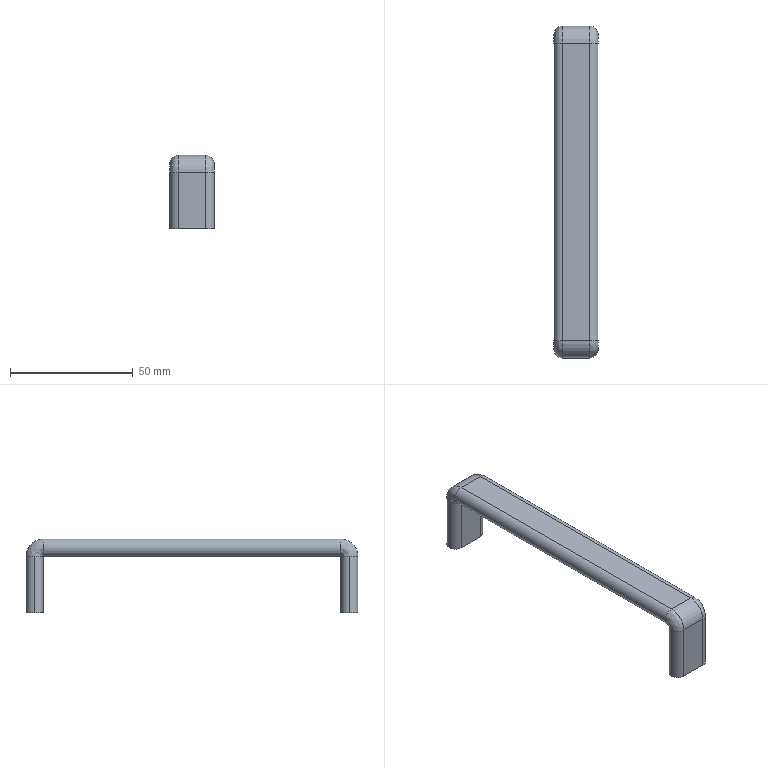Part | SolidWorks | features BaseBody 1 | 1 solid | 30 faces | box 18 x 135 x 30 mm | volume 20354 mm3 | cylinder 14 | plane 8 | cone 4 | spline 4 | commonest cylinder face diameters 7 x8 3.3 x4 14 x2
STEP:
#1=CARTESIAN_POINT('',(-9.,-64.,23.));
#2=VERTEX_POINT('',#1);
#3=CARTESIAN_POINT('',(-5.5,-67.5,23.));
#4=VERTEX_POINT('',#3);
#5=CARTESIAN_POINT('',(-5.5,-64.,23.));
#6=DIRECTION('',(0.,0.,1.));
#7=DIRECTION('',(0.,-1.,0.));
#8=AXIS2_PLACEMENT_3D('',#5,#6,#7);
#9=CIRCLE('',#8,3.5);
#10=EDGE_CURVE('',#2,#4,#9,.T.);
#11=ORIENTED_EDGE('',*,*,#10,.F.);
#12=CARTESIAN_POINT('',(-9.,-64.,0.));
#13=VERTEX_POINT('',#12);
#14=CARTESIAN_POINT('',(-9.,-64.,23.));
#15=DIRECTION('',(0.,0.,-1.));
#16=VECTOR('',#15,1000.);
#17=LINE('',#14,#16);
#18=EDGE_CURVE('',#2,#13,#17,.T.);
#19=ORIENTED_EDGE('',*,*,#18,.T.);
#20=CARTESIAN_POINT('',(-5.5,-67.5,0.));
#21=VERTEX_POINT('',#20);
#22=CARTESIAN_POINT('',(-5.5,-64.,0.));
#23=DIRECTION('',(0.,0.,1.));
#24=DIRECTION('',(-1.,0.,0.));
#25=AXIS2_PLACEMENT_3D('',#22,#23,#24);
#26=CIRCLE('',#25,3.5);
#27=EDGE_CURVE('',#13,#21,#26,.T.);
#28=ORIENTED_EDGE('',*,*,#27,.T.);
#29=CARTESIAN_POINT('',(-5.5,-67.5,23.));
#30=DIRECTION('',(0.,0.,1.));
#31=VECTOR('',#30,1000.);
#32=LINE('',#29,#31);
#33=EDGE_CURVE('',#21,#4,#32,.T.);
#34=ORIENTED_EDGE('',*,*,#33,.T.);
#35=EDGE_LOOP('',(#11,#19,#28,#34));
#36=FACE_OUTER_BOUND('',#35,.T.);
#37=CARTESIAN_POINT('',(-5.5,-64.,23.));
#38=DIRECTION('',(0.,0.,-1.));
#39=DIRECTION('',(-1.,0.,0.));
#40=AXIS2_PLACEMENT_3D('',#37,#38,#39);
#41=CYLINDRICAL_SURFACE('',#40,3.5);
#42=ADVANCED_FACE('',(#36),#41,.T.);
#43=CARTESIAN_POINT('',(-9.,64.,23.));
#44=VERTEX_POINT('',#43);
#45=CARTESIAN_POINT('',(-5.5,60.5,23.));
#46=VERTEX_POINT('',#45);
#47=CARTESIAN_POINT('',(-5.5,64.,23.));
#48=DIRECTION('',(0.,0.,1.));
#49=DIRECTION('',(0.,1.,0.));
#50=AXIS2_PLACEMENT_3D('',#47,#48,#49);
#51=CIRCLE('',#50,3.5);
#52=EDGE_CURVE('',#44,#46,#51,.T.);
#53=ORIENTED_EDGE('',*,*,#52,.F.);
#54=CARTESIAN_POINT('',(-9.,64.,0.));
#55=VERTEX_POINT('',#54);
#56=CARTESIAN_POINT('',(-9.,64.,23.));
#57=DIRECTION('',(0.,0.,-1.));
#58=VECTOR('',#57,1000.);
#59=LINE('',#56,#58);
#60=EDGE_CURVE('',#44,#55,#59,.T.);
#61=ORIENTED_EDGE('',*,*,#60,.T.);
#62=CARTESIAN_POINT('',(-5.5,60.5,0.));
#63=VERTEX_POINT('',#62);
#64=CARTESIAN_POINT('',(-5.5,64.,0.));
#65=DIRECTION('',(0.,0.,1.));
#66=DIRECTION('',(-1.,0.,0.));
#67=AXIS2_PLACEMENT_3D('',#64,#65,#66);
#68=CIRCLE('',#67,3.5);
#69=EDGE_CURVE('',#55,#63,#68,.T.);
#70=ORIENTED_EDGE('',*,*,#69,.T.);
#71=CARTESIAN_POINT('',(-5.5,60.5,23.));
#72=DIRECTION('',(0.,0.,1.));
#73=VECTOR('',#72,1000.);
#74=LINE('',#71,#73);
#75=EDGE_CURVE('',#63,#46,#74,.T.);
#76=ORIENTED_EDGE('',*,*,#75,.T.);
#77=EDGE_LOOP('',(#53,#61,#70,#76));
#78=FACE_OUTER_BOUND('',#77,.T.);
#79=CARTESIAN_POINT('',(-5.5,64.,23.));
#80=DIRECTION('',(0.,0.,-1.));
#81=DIRECTION('',(-1.,0.,0.));
#82=AXIS2_PLACEMENT_3D('',#79,#80,#81);
#83=CYLINDRICAL_SURFACE('',#82,3.5);
#84=ADVANCED_FACE('',(#78),#83,.T.);
#85=CARTESIAN_POINT('',(1.65,-64.,11.5));
#86=VERTEX_POINT('',#85);
#87=CARTESIAN_POINT('',(-1.65,-64.,11.5));
#88=VERTEX_POINT('',#87);
#89=CARTESIAN_POINT('',(0.,-64.,11.5));
#90=DIRECTION('',(0.,0.,-1.));
#91=DIRECTION('',(-1.,0.,0.));
#92=AXIS2_PLACEMENT_3D('',#89,#90,#91);
#93=CIRCLE('',#92,1.65);
#94=EDGE_CURVE('',#86,#88,#93,.T.);
#95=ORIENTED_EDGE('',*,*,#94,.F.);
#96=CARTESIAN_POINT('',(1.65,-64.,0.));
#97=VERTEX_POINT('',#96);
#98=CARTESIAN_POINT('',(1.65,-64.,0.));
#99=DIRECTION('',(0.,0.,-1.));
#100=VECTOR('',#99,1000.);
#101=LINE('',#98,#100);
#102=EDGE_CURVE('',#86,#97,#101,.T.);
#103=ORIENTED_EDGE('',*,*,#102,.T.);
#104=CARTESIAN_POINT('',(-1.65,-64.,0.));
#105=VERTEX_POINT('',#104);
#106=CARTESIAN_POINT('',(0.,-64.,0.));
#107=DIRECTION('',(0.,0.,1.));
#108=DIRECTION('',(-1.,0.,0.));
#109=AXIS2_PLACEMENT_3D('',#106,#107,#108);
#110=CIRCLE('',#109,1.65);
#111=EDGE_CURVE('',#105,#97,#110,.T.);
#112=ORIENTED_EDGE('',*,*,#111,.F.);
#113=CARTESIAN_POINT('',(-1.65,-64.,0.));
#114=DIRECTION('',(0.,0.,-1.));
#115=VECTOR('',#114,1000.);
#116=LINE('',#113,#115);
#117=EDGE_CURVE('',#88,#105,#116,.T.);
#118=ORIENTED_EDGE('',*,*,#117,.F.);
#119=EDGE_LOOP('',(#95,#103,#112,#118));
#120=FACE_OUTER_BOUND('',#119,.T.);
#121=CARTESIAN_POINT('',(0.,-64.,0.));
#122=DIRECTION('',(0.,0.,-1.));
#123=DIRECTION('',(-1.,0.,0.));
#124=AXIS2_PLACEMENT_3D('',#121,#122,#123);
#125=CYLINDRICAL_SURFACE('',#124,1.65);
#126=ADVANCED_FACE('',(#120),#125,.F.);
#127=CARTESIAN_POINT('',(1.65,64.,11.5));
#128=VERTEX_POINT('',#127);
#129=CARTESIAN_POINT('',(-1.65,64.,11.5));
#130=VERTEX_POINT('',#129);
#131=CARTESIAN_POINT('',(0.,64.,11.5));
#132=DIRECTION('',(0.,0.,-1.));
#133=DIRECTION('',(-1.,0.,0.));
#134=AXIS2_PLACEMENT_3D('',#131,#132,#133);
#135=CIRCLE('',#134,1.65);
#136=EDGE_CURVE('',#128,#130,#135,.T.);
#137=ORIENTED_EDGE('',*,*,#136,.F.);
#138=CARTESIAN_POINT('',(1.65,64.,0.));
#139=VERTEX_POINT('',#138);
#140=CARTESIAN_POINT('',(1.65,64.,0.));
#141=DIRECTION('',(0.,0.,-1.));
#142=VECTOR('',#141,1000.);
#143=LINE('',#140,#142);
#144=EDGE_CURVE('',#128,#139,#143,.T.);
#145=ORIENTED_EDGE('',*,*,#144,.T.);
#146=CARTESIAN_POINT('',(-1.65,64.,0.));
#147=VERTEX_POINT('',#146);
#148=CARTESIAN_POINT('',(0.,64.,0.));
#149=DIRECTION('',(0.,0.,-1.));
#150=DIRECTION('',(-1.,0.,0.));
#151=AXIS2_PLACEMENT_3D('',#148,#149,#150);
#152=CIRCLE('',#151,1.65);
#153=EDGE_CURVE('',#139,#147,#152,.T.);
#154=ORIENTED_EDGE('',*,*,#153,.T.);
#155=CARTESIAN_POINT('',(-1.65,64.,0.));
#156=DIRECTION('',(0.,0.,-1.));
#157=VECTOR('',#156,1000.);
#158=LINE('',#155,#157);
#159=EDGE_CURVE('',#130,#147,#158,.T.);
#160=ORIENTED_EDGE('',*,*,#159,.F.);
#161=EDGE_LOOP('',(#137,#145,#154,#160));
#162=FACE_OUTER_BOUND('',#161,.T.);
#163=CARTESIAN_POINT('',(0.,64.,0.));
#164=DIRECTION('',(0.,0.,-1.));
#165=DIRECTION('',(-1.,0.,0.));
#166=AXIS2_PLACEMENT_3D('',#163,#164,#165);
#167=CYLINDRICAL_SURFACE('',#166,1.65);
#168=ADVANCED_FACE('',(#162),#167,.F.);
#169=CARTESIAN_POINT('',(0.,-64.,12.491));
#170=VERTEX_POINT('',#169);
#171=CARTESIAN_POINT('',(-1.65,-64.,11.5));
#172=DIRECTION('',(-0.8572,0.,-0.515));
#173=VECTOR('',#172,1000.);
#174=LINE('',#171,#173);
#175=EDGE_CURVE('',#170,#88,#174,.T.);
#176=ORIENTED_EDGE('',*,*,#175,.F.);
#177=CARTESIAN_POINT('',(1.65,-64.,11.5));
#178=DIRECTION('',(0.8572,0.,-0.515));
#179=VECTOR('',#178,1000.);
#180=LINE('',#177,#179);
#181=EDGE_CURVE('',#170,#86,#180,.T.);
#182=ORIENTED_EDGE('',*,*,#181,.T.);
#183=ORIENTED_EDGE('',*,*,#94,.T.);
#184=EDGE_LOOP('',(#176,#182,#183));
#185=FACE_OUTER_BOUND('',#184,.T.);
#186=CARTESIAN_POINT('',(0.,-64.,11.5));
#187=DIRECTION('',(0.,0.,-1.));
#188=DIRECTION('',(-1.,0.,0.));
#189=AXIS2_PLACEMENT_3D('',#186,#187,#188);
#190=CONICAL_SURFACE('',#189,1.65,1.03);
#191=ADVANCED_FACE('',(#185),#190,.F.);
#192=CARTESIAN_POINT('',(0.,64.,12.491));
#193=VERTEX_POINT('',#192);
#194=CARTESIAN_POINT('',(-1.65,64.,11.5));
#195=DIRECTION('',(-0.8572,0.,-0.515));
#196=VECTOR('',#195,1000.);
#197=LINE('',#194,#196);
#198=EDGE_CURVE('',#193,#130,#197,.T.);
#199=ORIENTED_EDGE('',*,*,#198,.F.);
#200=CARTESIAN_POINT('',(1.65,64.,11.5));
#201=DIRECTION('',(0.8572,0.,-0.515));
#202=VECTOR('',#201,1000.);
#203=LINE('',#200,#202);
#204=EDGE_CURVE('',#193,#128,#203,.T.);
#205=ORIENTED_EDGE('',*,*,#204,.T.);
#206=ORIENTED_EDGE('',*,*,#136,.T.);
#207=EDGE_LOOP('',(#199,#205,#206));
#208=FACE_OUTER_BOUND('',#207,.T.);
#209=CARTESIAN_POINT('',(0.,64.,11.5));
#210=DIRECTION('',(0.,0.,-1.));
#211=DIRECTION('',(-1.,0.,0.));
#212=AXIS2_PLACEMENT_3D('',#209,#210,#211);
#213=CONICAL_SURFACE('',#212,1.65,1.03);
#214=ADVANCED_FACE('',(#208),#213,.F.);
#215=CARTESIAN_POINT('',(5.5,-60.5,23.));
#216=VERTEX_POINT('',#215);
#217=CARTESIAN_POINT('',(-5.5,-60.5,23.));
#218=VERTEX_POINT('',#217);
#219=CARTESIAN_POINT('',(-5.5,-60.5,23.));
#220=DIRECTION('',(-1.,0.,0.));
#221=VECTOR('',#220,1000.);
#222=LINE('',#219,#221);
#223=EDGE_CURVE('',#216,#218,#222,.T.);
#224=ORIENTED_EDGE('',*,*,#223,.T.);
#225=CARTESIAN_POINT('',(-5.5,60.5,23.));
#226=DIRECTION('',(0.,1.,0.));
#227=VECTOR('',#226,1000.);
#228=LINE('',#225,#227);
#229=EDGE_CURVE('',#218,#46,#228,.T.);
#230=ORIENTED_EDGE('',*,*,#229,.T.);
#231=CARTESIAN_POINT('',(5.5,60.5,23.));
#232=VERTEX_POINT('',#231);
#233=CARTESIAN_POINT('',(-5.5,60.5,23.));
#234=DIRECTION('',(1.,0.,0.));
#235=VECTOR('',#234,1000.);
#236=LINE('',#233,#235);
#237=EDGE_CURVE('',#46,#232,#236,.T.);
#238=ORIENTED_EDGE('',*,*,#237,.T.);
#239=CARTESIAN_POINT('',(5.5,60.5,23.));
#240=DIRECTION('',(0.,-1.,0.));
#241=VECTOR('',#240,1000.);
#242=LINE('',#239,#241);
#243=EDGE_CURVE('',#232,#216,#242,.T.);
#244=ORIENTED_EDGE('',*,*,#243,.T.);
#245=EDGE_LOOP('',(#224,#230,#238,#244));
#246=FACE_OUTER_BOUND('',#245,.T.);
#247=CARTESIAN_POINT('',(-5.5,60.5,23.));
#248=DIRECTION('',(0.,0.,-1.));
#249=DIRECTION('',(0.,1.,0.));
#250=AXIS2_PLACEMENT_3D('',#247,#248,#249);
#251=PLANE('',#250);
#252=ADVANCED_FACE('',(#246),#251,.T.);
#253=CARTESIAN_POINT('',(-5.5,-60.5,30.));
#254=VERTEX_POINT('',#253);
#255=CARTESIAN_POINT('',(-5.5,-60.5,26.5));
#256=DIRECTION('',(0.,1.,0.));
#257=DIRECTION('',(0.,0.,-1.));
#258=AXIS2_PLACEMENT_3D('',#255,#256,#257);
#259=CIRCLE('',#258,3.5);
#260=EDGE_CURVE('',#218,#254,#259,.T.);
#261=ORIENTED_EDGE('',*,*,#260,.T.);
#262=CARTESIAN_POINT('',(-5.5,60.5,30.));
#263=VERTEX_POINT('',#262);
#264=CARTESIAN_POINT('',(-5.5,60.5,30.));
#265=DIRECTION('',(0.,1.,0.));
#266=VECTOR('',#265,1000.);
#267=LINE('',#264,#266);
#268=EDGE_CURVE('',#254,#263,#267,.T.);
#269=ORIENTED_EDGE('',*,*,#268,.T.);
#270=CARTESIAN_POINT('',(-5.5,60.5,26.5));
#271=DIRECTION('',(0.,-1.,0.));
#272=DIRECTION('',(0.,0.,-1.));
#273=AXIS2_PLACEMENT_3D('',#270,#271,#272);
#274=CIRCLE('',#273,3.5);
#275=EDGE_CURVE('',#263,#46,#274,.T.);
#276=ORIENTED_EDGE('',*,*,#275,.T.);
#277=ORIENTED_EDGE('',*,*,#229,.F.);
#278=EDGE_LOOP('',(#261,#269,#276,#277));
#279=FACE_OUTER_BOUND('',#278,.T.);
#280=CARTESIAN_POINT('',(-5.5,60.5,26.5));
#281=DIRECTION('',(0.,-1.,0.));
#282=DIRECTION('',(0.,0.,-1.));
#283=AXIS2_PLACEMENT_3D('',#280,#281,#282);
#284=CYLINDRICAL_SURFACE('',#283,3.5);
#285=ADVANCED_FACE('',(#279),#284,.T.);
#286=CARTESIAN_POINT('',(5.5,-60.5,0.));
#287=VERTEX_POINT('',#286);
#288=CARTESIAN_POINT('',(-5.5,-60.5,0.));
#289=VERTEX_POINT('',#288);
#290=CARTESIAN_POINT('',(-5.5,-60.5,0.));
#291=DIRECTION('',(-1.,0.,0.));
#292=VECTOR('',#291,1000.);
#293=LINE('',#290,#292);
#294=EDGE_CURVE('',#287,#289,#293,.T.);
#295=ORIENTED_EDGE('',*,*,#294,.T.);
#296=CARTESIAN_POINT('',(-5.5,-60.5,23.));
#297=DIRECTION('',(0.,0.,1.));
#298=VECTOR('',#297,1000.);
#299=LINE('',#296,#298);
#300=EDGE_CURVE('',#289,#218,#299,.T.);
#301=ORIENTED_EDGE('',*,*,#300,.T.);
#302=ORIENTED_EDGE('',*,*,#223,.F.);
#303=CARTESIAN_POINT('',(5.5,-60.5,23.));
#304=DIRECTION('',(0.,0.,-1.));
#305=VECTOR('',#304,1000.);
#306=LINE('',#303,#305);
#307=EDGE_CURVE('',#216,#287,#306,.T.);
#308=ORIENTED_EDGE('',*,*,#307,.T.);
#309=EDGE_LOOP('',(#295,#301,#302,#308));
#310=FACE_OUTER_BOUND('',#309,.T.);
#311=CARTESIAN_POINT('',(-5.5,-60.5,23.));
#312=DIRECTION('',(0.,1.,0.));
#313=DIRECTION('',(0.,0.,1.));
#314=AXIS2_PLACEMENT_3D('',#311,#312,#313);
#315=PLANE('',#314);
#316=ADVANCED_FACE('',(#310),#315,.T.);
#317=CARTESIAN_POINT('',(5.5,-60.5,30.));
#318=VERTEX_POINT('',#317);
#319=CARTESIAN_POINT('',(5.5,-60.5,26.5));
#320=DIRECTION('',(0.,1.,0.));
#321=DIRECTION('',(0.,0.,-1.));
#322=AXIS2_PLACEMENT_3D('',#319,#320,#321);
#323=CIRCLE('',#322,3.5);
#324=EDGE_CURVE('',#318,#216,#323,.T.);
#325=ORIENTED_EDGE('',*,*,#324,.T.);
#326=ORIENTED_EDGE('',*,*,#243,.F.);
#327=CARTESIAN_POINT('',(5.5,60.5,30.));
#328=VERTEX_POINT('',#327);
#329=CARTESIAN_POINT('',(5.5,60.5,26.5));
#330=DIRECTION('',(0.,-1.,0.));
#331=DIRECTION('',(0.,0.,-1.));
#332=AXIS2_PLACEMENT_3D('',#329,#330,#331);
#333=CIRCLE('',#332,3.5);
#334=EDGE_CURVE('',#232,#328,#333,.T.);
#335=ORIENTED_EDGE('',*,*,#334,.T.);
#336=CARTESIAN_POINT('',(5.5,60.5,30.));
#337=DIRECTION('',(0.,-1.,0.));
#338=VECTOR('',#337,1000.);
#339=LINE('',#336,#338);
#340=EDGE_CURVE('',#328,#318,#339,.T.);
#341=ORIENTED_EDGE('',*,*,#340,.T.);
#342=EDGE_LOOP('',(#325,#326,#335,#341));
#343=FACE_OUTER_BOUND('',#342,.T.);
#344=CARTESIAN_POINT('',(5.5,60.5,26.5));
#345=DIRECTION('',(0.,-1.,0.));
#346=DIRECTION('',(0.,0.,-1.));
#347=AXIS2_PLACEMENT_3D('',#344,#345,#346);
#348=CYLINDRICAL_SURFACE('',#347,3.5);
#349=ADVANCED_FACE('',(#343),#348,.T.);
#350=CARTESIAN_POINT('',(5.5,60.5,0.));
#351=VERTEX_POINT('',#350);
#352=CARTESIAN_POINT('',(5.5,60.5,23.));
#353=DIRECTION('',(0.,0.,-1.));
#354=VECTOR('',#353,1000.);
#355=LINE('',#352,#354);
#356=EDGE_CURVE('',#232,#351,#355,.T.);
#357=ORIENTED_EDGE('',*,*,#356,.F.);
#358=ORIENTED_EDGE('',*,*,#237,.F.);
#359=ORIENTED_EDGE('',*,*,#75,.F.);
#360=CARTESIAN_POINT('',(-5.5,60.5,0.));
#361=DIRECTION('',(-1.,0.,0.));
#362=VECTOR('',#361,1000.);
#363=LINE('',#360,#362);
#364=EDGE_CURVE('',#351,#63,#363,.T.);
#365=ORIENTED_EDGE('',*,*,#364,.F.);
#366=EDGE_LOOP('',(#357,#358,#359,#365));
#367=FACE_OUTER_BOUND('',#366,.T.);
#368=CARTESIAN_POINT('',(-5.5,60.5,23.));
#369=DIRECTION('',(0.,1.,0.));
#370=DIRECTION('',(0.,0.,1.));
#371=AXIS2_PLACEMENT_3D('',#368,#369,#370);
#372=PLANE('',#371);
#373=ADVANCED_FACE('',(#367),#372,.F.);
#374=CARTESIAN_POINT('',(-5.5,-60.5,30.));
#375=DIRECTION('',(1.,0.,0.));
#376=VECTOR('',#375,1000.);
#377=LINE('',#374,#376);
#378=EDGE_CURVE('',#254,#318,#377,.T.);
#379=ORIENTED_EDGE('',*,*,#378,.T.);
#380=ORIENTED_EDGE('',*,*,#340,.F.);
#381=CARTESIAN_POINT('',(-5.5,60.5,30.));
#382=DIRECTION('',(-1.,0.,0.));
#383=VECTOR('',#382,1000.);
#384=LINE('',#381,#383);
#385=EDGE_CURVE('',#328,#263,#384,.T.);
#386=ORIENTED_EDGE('',*,*,#385,.T.);
#387=ORIENTED_EDGE('',*,*,#268,.F.);
#388=EDGE_LOOP('',(#379,#380,#386,#387));
#389=FACE_OUTER_BOUND('',#388,.T.);
#390=CARTESIAN_POINT('',(-5.5,60.5,30.));
#391=DIRECTION('',(0.,0.,1.));
#392=DIRECTION('',(0.,-1.,0.));
#393=AXIS2_PLACEMENT_3D('',#390,#391,#392);
#394=PLANE('',#393);
#395=ADVANCED_FACE('',(#389),#394,.T.);
#396=CARTESIAN_POINT('',(-5.5,-64.,23.));
#397=DIRECTION('',(0.,0.,1.));
#398=DIRECTION('',(0.,-1.,0.));
#399=AXIS2_PLACEMENT_3D('',#396,#397,#398);
#400=CIRCLE('',#399,3.5);
#401=EDGE_CURVE('',#218,#2,#400,.T.);
#402=ORIENTED_EDGE('',*,*,#401,.T.);
#403=ORIENTED_EDGE('',*,*,#10,.T.);
#404=CARTESIAN_POINT('',(-5.5,-60.5,23.));
#405=DIRECTION('',(-1.,0.,0.));
#406=DIRECTION('',(0.,0.,-1.));
#407=AXIS2_PLACEMENT_3D('',#404,#405,#406);
#408=CIRCLE('',#407,7.);
#409=EDGE_CURVE('',#4,#254,#408,.T.);
#410=ORIENTED_EDGE('',*,*,#409,.T.);
#411=ORIENTED_EDGE('',*,*,#260,.F.);
#412=EDGE_LOOP('',(#402,#403,#410,#411));
#413=FACE_OUTER_BOUND('',#412,.T.);
#414=CARTESIAN_POINT('',(-5.5,-60.5,30.));
#415=CARTESIAN_POINT('',(-5.5,-64.601,30.));
#416=CARTESIAN_POINT('',(-5.5,-67.5,27.101));
#417=CARTESIAN_POINT('',(-5.5,-67.5,23.));
#418=CARTESIAN_POINT('',(-12.5,-60.5,30.));
#419=CARTESIAN_POINT('',(-12.5,-64.601,30.));
#420=CARTESIAN_POINT('',(-12.5,-67.5,27.101));
#421=CARTESIAN_POINT('',(-12.5,-67.5,23.));
#422=CARTESIAN_POINT('',(-12.5,-60.5,23.));
#423=CARTESIAN_POINT('',(-12.5,-60.5,23.));
#424=CARTESIAN_POINT('',(-12.5,-60.5,23.));
#425=CARTESIAN_POINT('',(-12.5,-60.5,23.));
#426=CARTESIAN_POINT('',(-5.5,-60.5,23.));
#427=CARTESIAN_POINT('',(-5.5,-60.5,23.));
#428=CARTESIAN_POINT('',(-5.5,-60.5,23.));
#429=CARTESIAN_POINT('',(-5.5,-60.5,23.));
#430=(BOUNDED_SURFACE()B_SPLINE_SURFACE(3,3,((#414,#415,#416,#417),(#418,#419,#420,#421),(#422,#423,#424,#425),(#426,#427,#428,#429)),.UNSPECIFIED.,.F.,.F.,.F.)B_SPLINE_SURFACE_WITH_KNOTS((4,4),(4,4),(0.,1.),(0.,1.),.UNSPECIFIED.)GEOMETRIC_REPRESENTATION_ITEM()RATIONAL_B_SPLINE_SURFACE(((1.,0.8047,0.8047,1.),(0.3333,0.2682,0.2682,0.3333),(0.3333,0.2682,0.2682,0.3333),(1.,0.8047,0.8047,1.)))REPRESENTATION_ITEM('')SURFACE());
#431=ADVANCED_FACE('',(#413),#430,.T.);
#432=ORIENTED_EDGE('',*,*,#275,.F.);
#433=CARTESIAN_POINT('',(-5.5,67.5,23.));
#434=VERTEX_POINT('',#433);
#435=CARTESIAN_POINT('',(-5.5,60.5,23.));
#436=DIRECTION('',(-1.,0.,0.));
#437=DIRECTION('',(0.,0.,-1.));
#438=AXIS2_PLACEMENT_3D('',#435,#436,#437);
#439=CIRCLE('',#438,7.);
#440=EDGE_CURVE('',#263,#434,#439,.T.);
#441=ORIENTED_EDGE('',*,*,#440,.T.);
#442=CARTESIAN_POINT('',(-5.5,64.,23.));
#443=DIRECTION('',(0.,0.,1.));
#444=DIRECTION('',(0.,1.,0.));
#445=AXIS2_PLACEMENT_3D('',#442,#443,#444);
#446=CIRCLE('',#445,3.5);
#447=EDGE_CURVE('',#434,#44,#446,.T.);
#448=ORIENTED_EDGE('',*,*,#447,.T.);
#449=ORIENTED_EDGE('',*,*,#52,.T.);
#450=EDGE_LOOP('',(#432,#441,#448,#449));
#451=FACE_OUTER_BOUND('',#450,.T.);
#452=CARTESIAN_POINT('',(-5.5,67.5,23.));
#453=CARTESIAN_POINT('',(-5.5,67.5,27.101));
#454=CARTESIAN_POINT('',(-5.5,64.601,30.));
#455=CARTESIAN_POINT('',(-5.5,60.5,30.));
#456=CARTESIAN_POINT('',(-12.5,67.5,23.));
#457=CARTESIAN_POINT('',(-12.5,67.5,27.101));
#458=CARTESIAN_POINT('',(-12.5,64.601,30.));
#459=CARTESIAN_POINT('',(-12.5,60.5,30.));
#460=CARTESIAN_POINT('',(-12.5,60.5,23.));
#461=CARTESIAN_POINT('',(-12.5,60.5,23.));
#462=CARTESIAN_POINT('',(-12.5,60.5,23.));
#463=CARTESIAN_POINT('',(-12.5,60.5,23.));
#464=CARTESIAN_POINT('',(-5.5,60.5,23.));
#465=CARTESIAN_POINT('',(-5.5,60.5,23.));
#466=CARTESIAN_POINT('',(-5.5,60.5,23.));
#467=CARTESIAN_POINT('',(-5.5,60.5,23.));
#468=(BOUNDED_SURFACE()B_SPLINE_SURFACE(3,3,((#452,#453,#454,#455),(#456,#457,#458,#459),(#460,#461,#462,#463),(#464,#465,#466,#467)),.UNSPECIFIED.,.F.,.F.,.F.)B_SPLINE_SURFACE_WITH_KNOTS((4,4),(4,4),(0.,1.),(0.,1.),.UNSPECIFIED.)GEOMETRIC_REPRESENTATION_ITEM()RATIONAL_B_SPLINE_SURFACE(((1.,0.8047,0.8047,1.),(0.3333,0.2682,0.2682,0.3333),(0.3333,0.2682,0.2682,0.3333),(1.,0.8047,0.8047,1.)))REPRESENTATION_ITEM('')SURFACE());
#469=ADVANCED_FACE('',(#451),#468,.T.);
#470=ORIENTED_EDGE('',*,*,#18,.F.);
#471=ORIENTED_EDGE('',*,*,#401,.F.);
#472=ORIENTED_EDGE('',*,*,#300,.F.);
#473=CARTESIAN_POINT('',(-5.5,-64.,0.));
#474=DIRECTION('',(0.,0.,1.));
#475=DIRECTION('',(-1.,0.,0.));
#476=AXIS2_PLACEMENT_3D('',#473,#474,#475);
#477=CIRCLE('',#476,3.5);
#478=EDGE_CURVE('',#289,#13,#477,.T.);
#479=ORIENTED_EDGE('',*,*,#478,.T.);
#480=EDGE_LOOP('',(#470,#471,#472,#479));
#481=FACE_OUTER_BOUND('',#480,.T.);
#482=CARTESIAN_POINT('',(-5.5,-64.,23.));
#483=DIRECTION('',(0.,0.,-1.));
#484=DIRECTION('',(-1.,0.,0.));
#485=AXIS2_PLACEMENT_3D('',#482,#483,#484);
#486=CYLINDRICAL_SURFACE('',#485,3.5);
#487=ADVANCED_FACE('',(#481),#486,.T.);
#488=CARTESIAN_POINT('',(5.5,-67.5,0.));
#489=VERTEX_POINT('',#488);
#490=CARTESIAN_POINT('',(5.5,-64.,0.));
#491=DIRECTION('',(0.,0.,-1.));
#492=DIRECTION('',(-1.,0.,0.));
#493=AXIS2_PLACEMENT_3D('',#490,#491,#492);
#494=CIRCLE('',#493,3.5);
#495=EDGE_CURVE('',#287,#489,#494,.T.);
#496=ORIENTED_EDGE('',*,*,#495,.T.);
#497=CARTESIAN_POINT('',(-5.5,-67.5,0.));
#498=DIRECTION('',(-1.,0.,0.));
#499=VECTOR('',#498,1000.);
#500=LINE('',#497,#499);
#501=EDGE_CURVE('',#489,#21,#500,.T.);
#502=ORIENTED_EDGE('',*,*,#501,.T.);
#503=ORIENTED_EDGE('',*,*,#27,.F.);
#504=ORIENTED_EDGE('',*,*,#478,.F.);
#505=ORIENTED_EDGE('',*,*,#294,.F.);
#506=EDGE_LOOP('',(#496,#502,#503,#504,#505));
#507=FACE_OUTER_BOUND('',#506,.T.);
#508=ORIENTED_EDGE('',*,*,#111,.T.);
#509=CARTESIAN_POINT('',(0.,-64.,0.));
#510=DIRECTION('',(0.,0.,1.));
#511=DIRECTION('',(-1.,0.,0.));
#512=AXIS2_PLACEMENT_3D('',#509,#510,#511);
#513=CIRCLE('',#512,1.65);
#514=EDGE_CURVE('',#97,#105,#513,.T.);
#515=ORIENTED_EDGE('',*,*,#514,.T.);
#516=EDGE_LOOP('',(#508,#515));
#517=FACE_BOUND('',#516,.T.);
#518=CARTESIAN_POINT('',(-5.5,-64.,0.));
#519=DIRECTION('',(0.,0.,-1.));
#520=DIRECTION('',(0.,1.,0.));
#521=AXIS2_PLACEMENT_3D('',#518,#519,#520);
#522=PLANE('',#521);
#523=ADVANCED_FACE('',(#507,#517),#522,.T.);
#524=ORIENTED_EDGE('',*,*,#495,.F.);
#525=ORIENTED_EDGE('',*,*,#307,.F.);
#526=CARTESIAN_POINT('',(5.5,-67.5,23.));
#527=VERTEX_POINT('',#526);
#528=CARTESIAN_POINT('',(5.5,-64.,23.));
#529=DIRECTION('',(0.,0.,-1.));
#530=DIRECTION('',(-1.,0.,0.));
#531=AXIS2_PLACEMENT_3D('',#528,#529,#530);
#532=CIRCLE('',#531,3.5);
#533=EDGE_CURVE('',#216,#527,#532,.T.);
#534=ORIENTED_EDGE('',*,*,#533,.T.);
#535=CARTESIAN_POINT('',(5.5,-67.5,23.));
#536=DIRECTION('',(0.,0.,-1.));
#537=VECTOR('',#536,1000.);
#538=LINE('',#535,#537);
#539=EDGE_CURVE('',#527,#489,#538,.T.);
#540=ORIENTED_EDGE('',*,*,#539,.T.);
#541=EDGE_LOOP('',(#524,#525,#534,#540));
#542=FACE_OUTER_BOUND('',#541,.T.);
#543=CARTESIAN_POINT('',(5.5,-64.,23.));
#544=DIRECTION('',(0.,0.,-1.));
#545=DIRECTION('',(-1.,0.,0.));
#546=AXIS2_PLACEMENT_3D('',#543,#544,#545);
#547=CYLINDRICAL_SURFACE('',#546,3.5);
#548=ADVANCED_FACE('',(#542),#547,.T.);
#549=CARTESIAN_POINT('',(5.5,-60.5,23.));
#550=DIRECTION('',(1.,0.,0.));
#551=DIRECTION('',(0.,0.,-1.));
#552=AXIS2_PLACEMENT_3D('',#549,#550,#551);
#553=CIRCLE('',#552,7.);
#554=EDGE_CURVE('',#318,#527,#553,.T.);
#555=ORIENTED_EDGE('',*,*,#554,.T.);
#556=ORIENTED_EDGE('',*,*,#533,.F.);
#557=ORIENTED_EDGE('',*,*,#324,.F.);
#558=EDGE_LOOP('',(#555,#556,#557));
#559=FACE_OUTER_BOUND('',#558,.T.);
#560=CARTESIAN_POINT('',(5.5,-60.5,23.));
#561=CARTESIAN_POINT('',(5.5,-60.5,23.));
#562=CARTESIAN_POINT('',(5.5,-60.5,23.));
#563=CARTESIAN_POINT('',(5.5,-60.5,23.));
#564=CARTESIAN_POINT('',(5.5,-60.5,23.));
#565=CARTESIAN_POINT('',(5.5,-60.5,23.));
#566=CARTESIAN_POINT('',(5.5,-60.5,23.));
#567=CARTESIAN_POINT('',(12.5,-60.5,23.));
#568=CARTESIAN_POINT('',(12.5,-60.5,23.));
#569=CARTESIAN_POINT('',(12.5,-60.5,23.));
#570=CARTESIAN_POINT('',(12.5,-60.5,23.));
#571=CARTESIAN_POINT('',(12.5,-60.5,23.));
#572=CARTESIAN_POINT('',(12.5,-60.5,23.));
#573=CARTESIAN_POINT('',(12.5,-60.5,23.));
#574=CARTESIAN_POINT('',(12.5,-60.5,16.));
#575=CARTESIAN_POINT('',(12.5,-46.5,16.));
#576=CARTESIAN_POINT('',(12.5,-46.5,30.));
#577=CARTESIAN_POINT('',(12.5,-60.5,30.));
#578=CARTESIAN_POINT('',(12.5,-74.5,30.));
#579=CARTESIAN_POINT('',(12.5,-74.5,16.));
#580=CARTESIAN_POINT('',(12.5,-60.5,16.));
#581=CARTESIAN_POINT('',(5.5,-60.5,16.));
#582=CARTESIAN_POINT('',(5.5,-46.5,16.));
#583=CARTESIAN_POINT('',(5.5,-46.5,30.));
#584=CARTESIAN_POINT('',(5.5,-60.5,30.));
#585=CARTESIAN_POINT('',(5.5,-74.5,30.));
#586=CARTESIAN_POINT('',(5.5,-74.5,16.));
#587=CARTESIAN_POINT('',(5.5,-60.5,16.));
#588=CARTESIAN_POINT('',(-1.5,-60.5,16.));
#589=CARTESIAN_POINT('',(-1.5,-46.5,16.));
#590=CARTESIAN_POINT('',(-1.5,-46.5,30.));
#591=CARTESIAN_POINT('',(-1.5,-60.5,30.));
#592=CARTESIAN_POINT('',(-1.5,-74.5,30.));
#593=CARTESIAN_POINT('',(-1.5,-74.5,16.));
#594=CARTESIAN_POINT('',(-1.5,-60.5,16.));
#595=CARTESIAN_POINT('',(-1.5,-60.5,23.));
#596=CARTESIAN_POINT('',(-1.5,-60.5,23.));
#597=CARTESIAN_POINT('',(-1.5,-60.5,23.));
#598=CARTESIAN_POINT('',(-1.5,-60.5,23.));
#599=CARTESIAN_POINT('',(-1.5,-60.5,23.));
#600=CARTESIAN_POINT('',(-1.5,-60.5,23.));
#601=CARTESIAN_POINT('',(-1.5,-60.5,23.));
#602=CARTESIAN_POINT('',(5.5,-60.5,23.));
#603=CARTESIAN_POINT('',(5.5,-60.5,23.));
#604=CARTESIAN_POINT('',(5.5,-60.5,23.));
#605=CARTESIAN_POINT('',(5.5,-60.5,23.));
#606=CARTESIAN_POINT('',(5.5,-60.5,23.));
#607=CARTESIAN_POINT('',(5.5,-60.5,23.));
#608=CARTESIAN_POINT('',(5.5,-60.5,23.));
#609=(BOUNDED_SURFACE()B_SPLINE_SURFACE(3,3,((#560,#561,#562,#563,#564,#565,#566),(#567,#568,#569,#570,#571,#572,#573),(#574,#575,#576,#577,#578,#579,#580),(#581,#582,#583,#584,#585,#586,#587),(#588,#589,#590,#591,#592,#593,#594),(#595,#596,#597,#598,#599,#600,#601),(#602,#603,#604,#605,#606,#607,#608)),.UNSPECIFIED.,.T.,.T.,.F.)B_SPLINE_SURFACE_WITH_KNOTS((4,3,4),(4,3,4),(0.,0.5,1.),(0.,0.5,1.),.UNSPECIFIED.)GEOMETRIC_REPRESENTATION_ITEM()RATIONAL_B_SPLINE_SURFACE(((1.,0.3333,0.3333,1.,0.3333,0.3333,1.),(0.3333,0.1111,0.1111,0.3333,0.1111,0.1111,0.3333),(0.3333,0.1111,0.1111,0.3333,0.1111,0.1111,0.3333),(1.,0.3333,0.3333,1.,0.3333,0.3333,1.),(0.3333,0.1111,0.1111,0.3333,0.1111,0.1111,0.3333),(0.3333,0.1111,0.1111,0.3333,0.1111,0.1111,0.3333),(1.,0.3333,0.3333,1.,0.3333,0.3333,1.)))REPRESENTATION_ITEM('')SURFACE());
#610=ADVANCED_FACE('',(#559),#609,.T.);
#611=CARTESIAN_POINT('',(5.5,67.5,23.));
#612=VERTEX_POINT('',#611);
#613=CARTESIAN_POINT('',(5.5,60.5,23.));
#614=DIRECTION('',(1.,0.,0.));
#615=DIRECTION('',(0.,0.,-1.));
#616=AXIS2_PLACEMENT_3D('',#613,#614,#615);
#617=CIRCLE('',#616,7.);
#618=EDGE_CURVE('',#612,#328,#617,.T.);
#619=ORIENTED_EDGE('',*,*,#618,.T.);
#620=ORIENTED_EDGE('',*,*,#334,.F.);
#621=CARTESIAN_POINT('',(5.5,64.,23.));
#622=DIRECTION('',(0.,0.,1.));
#623=DIRECTION('',(0.,1.,0.));
#624=AXIS2_PLACEMENT_3D('',#621,#622,#623);
#625=CIRCLE('',#624,3.5);
#626=EDGE_CURVE('',#232,#612,#625,.T.);
#627=ORIENTED_EDGE('',*,*,#626,.T.);
#628=EDGE_LOOP('',(#619,#620,#627));
#629=FACE_OUTER_BOUND('',#628,.T.);
#630=CARTESIAN_POINT('',(5.5,60.5,23.));
#631=CARTESIAN_POINT('',(5.5,60.5,23.));
#632=CARTESIAN_POINT('',(5.5,60.5,23.));
#633=CARTESIAN_POINT('',(5.5,60.5,23.));
#634=CARTESIAN_POINT('',(5.5,60.5,23.));
#635=CARTESIAN_POINT('',(5.5,60.5,23.));
#636=CARTESIAN_POINT('',(5.5,60.5,23.));
#637=CARTESIAN_POINT('',(12.5,60.5,23.));
#638=CARTESIAN_POINT('',(12.5,60.5,23.));
#639=CARTESIAN_POINT('',(12.5,60.5,23.));
#640=CARTESIAN_POINT('',(12.5,60.5,23.));
#641=CARTESIAN_POINT('',(12.5,60.5,23.));
#642=CARTESIAN_POINT('',(12.5,60.5,23.));
#643=CARTESIAN_POINT('',(12.5,60.5,23.));
#644=CARTESIAN_POINT('',(12.5,60.5,16.));
#645=CARTESIAN_POINT('',(12.5,74.5,16.));
#646=CARTESIAN_POINT('',(12.5,74.5,30.));
#647=CARTESIAN_POINT('',(12.5,60.5,30.));
#648=CARTESIAN_POINT('',(12.5,46.5,30.));
#649=CARTESIAN_POINT('',(12.5,46.5,16.));
#650=CARTESIAN_POINT('',(12.5,60.5,16.));
#651=CARTESIAN_POINT('',(5.5,60.5,16.));
#652=CARTESIAN_POINT('',(5.5,74.5,16.));
#653=CARTESIAN_POINT('',(5.5,74.5,30.));
#654=CARTESIAN_POINT('',(5.5,60.5,30.));
#655=CARTESIAN_POINT('',(5.5,46.5,30.));
#656=CARTESIAN_POINT('',(5.5,46.5,16.));
#657=CARTESIAN_POINT('',(5.5,60.5,16.));
#658=CARTESIAN_POINT('',(-1.5,60.5,16.));
#659=CARTESIAN_POINT('',(-1.5,74.5,16.));
#660=CARTESIAN_POINT('',(-1.5,74.5,30.));
#661=CARTESIAN_POINT('',(-1.5,60.5,30.));
#662=CARTESIAN_POINT('',(-1.5,46.5,30.));
#663=CARTESIAN_POINT('',(-1.5,46.5,16.));
#664=CARTESIAN_POINT('',(-1.5,60.5,16.));
#665=CARTESIAN_POINT('',(-1.5,60.5,23.));
#666=CARTESIAN_POINT('',(-1.5,60.5,23.));
#667=CARTESIAN_POINT('',(-1.5,60.5,23.));
#668=CARTESIAN_POINT('',(-1.5,60.5,23.));
#669=CARTESIAN_POINT('',(-1.5,60.5,23.));
#670=CARTESIAN_POINT('',(-1.5,60.5,23.));
#671=CARTESIAN_POINT('',(-1.5,60.5,23.));
#672=CARTESIAN_POINT('',(5.5,60.5,23.));
#673=CARTESIAN_POINT('',(5.5,60.5,23.));
#674=CARTESIAN_POINT('',(5.5,60.5,23.));
#675=CARTESIAN_POINT('',(5.5,60.5,23.));
#676=CARTESIAN_POINT('',(5.5,60.5,23.));
#677=CARTESIAN_POINT('',(5.5,60.5,23.));
#678=CARTESIAN_POINT('',(5.5,60.5,23.));
#679=(BOUNDED_SURFACE()B_SPLINE_SURFACE(3,3,((#630,#631,#632,#633,#634,#635,#636),(#637,#638,#639,#640,#641,#642,#643),(#644,#645,#646,#647,#648,#649,#650),(#651,#652,#653,#654,#655,#656,#657),(#658,#659,#660,#661,#662,#663,#664),(#665,#666,#667,#668,#669,#670,#671),(#672,#673,#674,#675,#676,#677,#678)),.UNSPECIFIED.,.T.,.T.,.F.)B_SPLINE_SURFACE_WITH_KNOTS((4,3,4),(4,3,4),(0.,0.5,1.),(0.,0.5,1.),.UNSPECIFIED.)GEOMETRIC_REPRESENTATION_ITEM()RATIONAL_B_SPLINE_SURFACE(((1.,0.3333,0.3333,1.,0.3333,0.3333,1.),(0.3333,0.1111,0.1111,0.3333,0.1111,0.1111,0.3333),(0.3333,0.1111,0.1111,0.3333,0.1111,0.1111,0.3333),(1.,0.3333,0.3333,1.,0.3333,0.3333,1.),(0.3333,0.1111,0.1111,0.3333,0.1111,0.1111,0.3333),(0.3333,0.1111,0.1111,0.3333,0.1111,0.1111,0.3333),(1.,0.3333,0.3333,1.,0.3333,0.3333,1.)))REPRESENTATION_ITEM('')SURFACE());
#680=ADVANCED_FACE('',(#629),#679,.T.);
#681=CARTESIAN_POINT('',(5.5,67.5,0.));
#682=VERTEX_POINT('',#681);
#683=CARTESIAN_POINT('',(-5.5,67.5,0.));
#684=VERTEX_POINT('',#683);
#685=CARTESIAN_POINT('',(-5.5,67.5,0.));
#686=DIRECTION('',(-1.,0.,0.));
#687=VECTOR('',#686,1000.);
#688=LINE('',#685,#687);
#689=EDGE_CURVE('',#682,#684,#688,.T.);
#690=ORIENTED_EDGE('',*,*,#689,.F.);
#691=CARTESIAN_POINT('',(5.5,64.,0.));
#692=DIRECTION('',(0.,0.,1.));
#693=DIRECTION('',(-1.,0.,0.));
#694=AXIS2_PLACEMENT_3D('',#691,#692,#693);
#695=CIRCLE('',#694,3.5);
#696=EDGE_CURVE('',#351,#682,#695,.T.);
#697=ORIENTED_EDGE('',*,*,#696,.F.);
#698=ORIENTED_EDGE('',*,*,#364,.T.);
#699=ORIENTED_EDGE('',*,*,#69,.F.);
#700=CARTESIAN_POINT('',(-5.5,64.,0.));
#701=DIRECTION('',(0.,0.,1.));
#702=DIRECTION('',(-1.,0.,0.));
#703=AXIS2_PLACEMENT_3D('',#700,#701,#702);
#704=CIRCLE('',#703,3.5);
#705=EDGE_CURVE('',#684,#55,#704,.T.);
#706=ORIENTED_EDGE('',*,*,#705,.F.);
#707=EDGE_LOOP('',(#690,#697,#698,#699,#706));
#708=FACE_OUTER_BOUND('',#707,.T.);
#709=CARTESIAN_POINT('',(0.,64.,0.));
#710=DIRECTION('',(0.,0.,-1.));
#711=DIRECTION('',(-1.,0.,0.));
#712=AXIS2_PLACEMENT_3D('',#709,#710,#711);
#713=CIRCLE('',#712,1.65);
#714=EDGE_CURVE('',#147,#139,#713,.T.);
#715=ORIENTED_EDGE('',*,*,#714,.F.);
#716=ORIENTED_EDGE('',*,*,#153,.F.);
#717=EDGE_LOOP('',(#715,#716));
#718=FACE_BOUND('',#717,.T.);
#719=CARTESIAN_POINT('',(-5.5,64.,0.));
#720=DIRECTION('',(0.,0.,1.));
#721=DIRECTION('',(1.,0.,0.));
#722=AXIS2_PLACEMENT_3D('',#719,#720,#721);
#723=PLANE('',#722);
#724=ADVANCED_FACE('',(#708,#718),#723,.F.);
#725=ORIENTED_EDGE('',*,*,#626,.F.);
#726=ORIENTED_EDGE('',*,*,#356,.T.);
#727=ORIENTED_EDGE('',*,*,#696,.T.);
#728=CARTESIAN_POINT('',(5.5,67.5,23.));
#729=DIRECTION('',(0.,0.,1.));
#730=VECTOR('',#729,1000.);
#731=LINE('',#728,#730);
#732=EDGE_CURVE('',#682,#612,#731,.T.);
#733=ORIENTED_EDGE('',*,*,#732,.T.);
#734=EDGE_LOOP('',(#725,#726,#727,#733));
#735=FACE_OUTER_BOUND('',#734,.T.);
#736=CARTESIAN_POINT('',(5.5,64.,23.));
#737=DIRECTION('',(0.,0.,-1.));
#738=DIRECTION('',(-1.,0.,0.));
#739=AXIS2_PLACEMENT_3D('',#736,#737,#738);
#740=CYLINDRICAL_SURFACE('',#739,3.5);
#741=ADVANCED_FACE('',(#735),#740,.T.);
#742=ORIENTED_EDGE('',*,*,#60,.F.);
#743=ORIENTED_EDGE('',*,*,#447,.F.);
#744=CARTESIAN_POINT('',(-5.5,67.5,23.));
#745=DIRECTION('',(0.,0.,-1.));
#746=VECTOR('',#745,1000.);
#747=LINE('',#744,#746);
#748=EDGE_CURVE('',#434,#684,#747,.T.);
#749=ORIENTED_EDGE('',*,*,#748,.T.);
#750=ORIENTED_EDGE('',*,*,#705,.T.);
#751=EDGE_LOOP('',(#742,#743,#749,#750));
#752=FACE_OUTER_BOUND('',#751,.T.);
#753=CARTESIAN_POINT('',(-5.5,64.,23.));
#754=DIRECTION('',(0.,0.,-1.));
#755=DIRECTION('',(-1.,0.,0.));
#756=AXIS2_PLACEMENT_3D('',#753,#754,#755);
#757=CYLINDRICAL_SURFACE('',#756,3.5);
#758=ADVANCED_FACE('',(#752),#757,.T.);
#759=CARTESIAN_POINT('',(0.,-67.5,23.));
#760=DIRECTION('',(1.,0.,0.));
#761=VECTOR('',#760,1000.);
#762=LINE('',#759,#761);
#763=EDGE_CURVE('',#4,#527,#762,.T.);
#764=ORIENTED_EDGE('',*,*,#763,.T.);
#765=ORIENTED_EDGE('',*,*,#554,.F.);
#766=ORIENTED_EDGE('',*,*,#378,.F.);
#767=ORIENTED_EDGE('',*,*,#409,.F.);
#768=EDGE_LOOP('',(#764,#765,#766,#767));
#769=FACE_OUTER_BOUND('',#768,.T.);
#770=CARTESIAN_POINT('',(0.,-60.5,23.));
#771=DIRECTION('',(1.,0.,0.));
#772=DIRECTION('',(0.,0.,-1.));
#773=AXIS2_PLACEMENT_3D('',#770,#771,#772);
#774=CYLINDRICAL_SURFACE('',#773,7.);
#775=ADVANCED_FACE('',(#769),#774,.T.);
#776=ORIENTED_EDGE('',*,*,#385,.F.);
#777=ORIENTED_EDGE('',*,*,#618,.F.);
#778=CARTESIAN_POINT('',(0.,67.5,23.));
#779=DIRECTION('',(-1.,0.,0.));
#780=VECTOR('',#779,1000.);
#781=LINE('',#778,#780);
#782=EDGE_CURVE('',#612,#434,#781,.T.);
#783=ORIENTED_EDGE('',*,*,#782,.T.);
#784=ORIENTED_EDGE('',*,*,#440,.F.);
#785=EDGE_LOOP('',(#776,#777,#783,#784));
#786=FACE_OUTER_BOUND('',#785,.T.);
#787=CARTESIAN_POINT('',(0.,60.5,23.));
#788=DIRECTION('',(1.,0.,0.));
#789=DIRECTION('',(0.,0.,-1.));
#790=AXIS2_PLACEMENT_3D('',#787,#788,#789);
#791=CYLINDRICAL_SURFACE('',#790,7.);
#792=ADVANCED_FACE('',(#786),#791,.T.);
#793=ORIENTED_EDGE('',*,*,#501,.F.);
#794=ORIENTED_EDGE('',*,*,#539,.F.);
#795=ORIENTED_EDGE('',*,*,#763,.F.);
#796=ORIENTED_EDGE('',*,*,#33,.F.);
#797=EDGE_LOOP('',(#793,#794,#795,#796));
#798=FACE_OUTER_BOUND('',#797,.T.);
#799=CARTESIAN_POINT('',(-5.5,-67.5,23.));
#800=DIRECTION('',(0.,-1.,0.));
#801=DIRECTION('',(0.,0.,-1.));
#802=AXIS2_PLACEMENT_3D('',#799,#800,#801);
#803=PLANE('',#802);
#804=ADVANCED_FACE('',(#798),#803,.T.);
#805=ORIENTED_EDGE('',*,*,#102,.F.);
#806=CARTESIAN_POINT('',(0.,-64.,11.5));
#807=DIRECTION('',(0.,0.,-1.));
#808=DIRECTION('',(-1.,0.,0.));
#809=AXIS2_PLACEMENT_3D('',#806,#807,#808);
#810=CIRCLE('',#809,1.65);
#811=EDGE_CURVE('',#88,#86,#810,.T.);
#812=ORIENTED_EDGE('',*,*,#811,.F.);
#813=ORIENTED_EDGE('',*,*,#117,.T.);
#814=ORIENTED_EDGE('',*,*,#514,.F.);
#815=EDGE_LOOP('',(#805,#812,#813,#814));
#816=FACE_OUTER_BOUND('',#815,.T.);
#817=CARTESIAN_POINT('',(0.,-64.,0.));
#818=DIRECTION('',(0.,0.,-1.));
#819=DIRECTION('',(-1.,0.,0.));
#820=AXIS2_PLACEMENT_3D('',#817,#818,#819);
#821=CYLINDRICAL_SURFACE('',#820,1.65);
#822=ADVANCED_FACE('',(#816),#821,.F.);
#823=ORIENTED_EDGE('',*,*,#748,.F.);
#824=ORIENTED_EDGE('',*,*,#782,.F.);
#825=ORIENTED_EDGE('',*,*,#732,.F.);
#826=ORIENTED_EDGE('',*,*,#689,.T.);
#827=EDGE_LOOP('',(#823,#824,#825,#826));
#828=FACE_OUTER_BOUND('',#827,.T.);
#829=CARTESIAN_POINT('',(-5.5,67.5,23.));
#830=DIRECTION('',(0.,-1.,0.));
#831=DIRECTION('',(0.,0.,-1.));
#832=AXIS2_PLACEMENT_3D('',#829,#830,#831);
#833=PLANE('',#832);
#834=ADVANCED_FACE('',(#828),#833,.F.);
#835=ORIENTED_EDGE('',*,*,#144,.F.);
#836=CARTESIAN_POINT('',(0.,64.,11.5));
#837=DIRECTION('',(0.,0.,-1.));
#838=DIRECTION('',(-1.,0.,0.));
#839=AXIS2_PLACEMENT_3D('',#836,#837,#838);
#840=CIRCLE('',#839,1.65);
#841=EDGE_CURVE('',#130,#128,#840,.T.);
#842=ORIENTED_EDGE('',*,*,#841,.F.);
#843=ORIENTED_EDGE('',*,*,#159,.T.);
#844=ORIENTED_EDGE('',*,*,#714,.T.);
#845=EDGE_LOOP('',(#835,#842,#843,#844));
#846=FACE_OUTER_BOUND('',#845,.T.);
#847=CARTESIAN_POINT('',(0.,64.,0.));
#848=DIRECTION('',(0.,0.,-1.));
#849=DIRECTION('',(-1.,0.,0.));
#850=AXIS2_PLACEMENT_3D('',#847,#848,#849);
#851=CYLINDRICAL_SURFACE('',#850,1.65);
#852=ADVANCED_FACE('',(#846),#851,.F.);
#853=ORIENTED_EDGE('',*,*,#181,.F.);
#854=ORIENTED_EDGE('',*,*,#175,.T.);
#855=ORIENTED_EDGE('',*,*,#811,.T.);
#856=EDGE_LOOP('',(#853,#854,#855));
#857=FACE_OUTER_BOUND('',#856,.T.);
#858=CARTESIAN_POINT('',(0.,-64.,11.5));
#859=DIRECTION('',(0.,0.,-1.));
#860=DIRECTION('',(-1.,0.,0.));
#861=AXIS2_PLACEMENT_3D('',#858,#859,#860);
#862=CONICAL_SURFACE('',#861,1.65,1.03);
#863=ADVANCED_FACE('',(#857),#862,.F.);
#864=ORIENTED_EDGE('',*,*,#204,.F.);
#865=ORIENTED_EDGE('',*,*,#198,.T.);
#866=ORIENTED_EDGE('',*,*,#841,.T.);
#867=EDGE_LOOP('',(#864,#865,#866));
#868=FACE_OUTER_BOUND('',#867,.T.);
#869=CARTESIAN_POINT('',(0.,64.,11.5));
#870=DIRECTION('',(0.,0.,-1.));
#871=DIRECTION('',(-1.,0.,0.));
#872=AXIS2_PLACEMENT_3D('',#869,#870,#871);
#873=CONICAL_SURFACE('',#872,1.65,1.03);
#874=ADVANCED_FACE('',(#868),#873,.F.);
#875=CLOSED_SHELL('',(#42,#84,#126,#168,#191,#214,#252,#285,#316,#349,#373,#395,#431,#469,#487,#523,#548,#610,#680,#724,#741,#758,#775,#792,#804,#822,#834,#852,#863,#874));
#876=MANIFOLD_SOLID_BREP('',#875);
#877=CARTESIAN_POINT('',(0.,0.,0.));
#878=DIRECTION('',(0.,0.,1.));
#879=DIRECTION('',(1.,0.,0.));
#880=AXIS2_PLACEMENT_3D('',#877,#878,#879);
#881=(LENGTH_UNIT()NAMED_UNIT(*)SI_UNIT(.MILLI.,.METRE.));
#882=UNCERTAINTY_MEASURE_WITH_UNIT(LENGTH_MEASURE(0.00001),#881,'','');
#883=(NAMED_UNIT(*)PLANE_ANGLE_UNIT()SI_UNIT($,.RADIAN.));
#884=(NAMED_UNIT(*)SI_UNIT($,.STERADIAN.)SOLID_ANGLE_UNIT());
#885=(GEOMETRIC_REPRESENTATION_CONTEXT(3)GLOBAL_UNCERTAINTY_ASSIGNED_CONTEXT((#882))GLOBAL_UNIT_ASSIGNED_CONTEXT((#881,#883,#884))REPRESENTATION_CONTEXT('',''));
#886=ADVANCED_BREP_SHAPE_REPRESENTATION('',(#876,#880),#885);